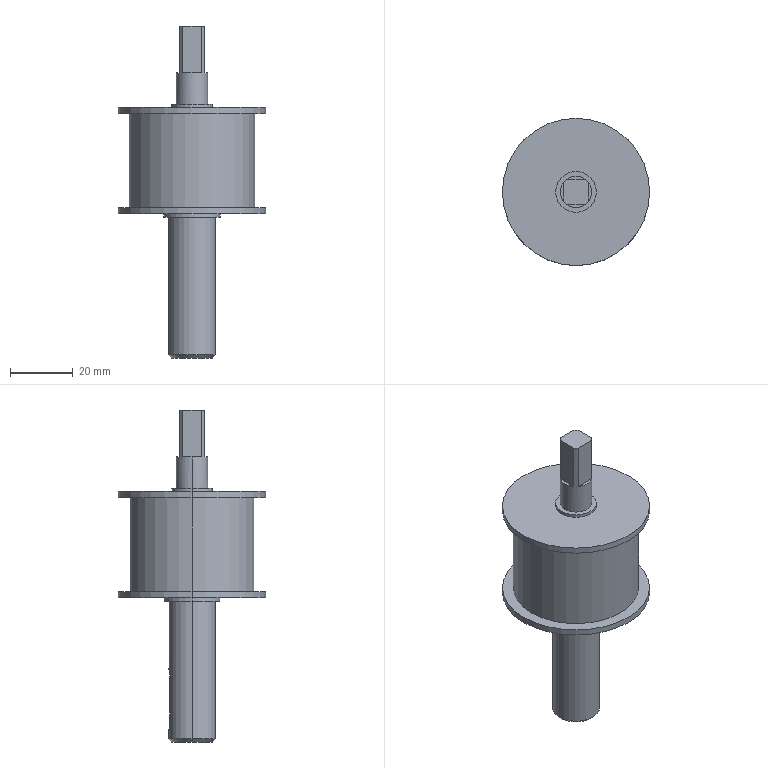Part | STEP file | (PA01.001.LX006) Drive Wheel B | 1 solid | 38 faces | box 47 x 47 x 106 mm | volume 54403 mm3 | plane 19 | cylinder 17 | cone 2 | commonest cylinder face diameters 47 x4 5 x3 10 x2 13 x2 15 x2 18 x2